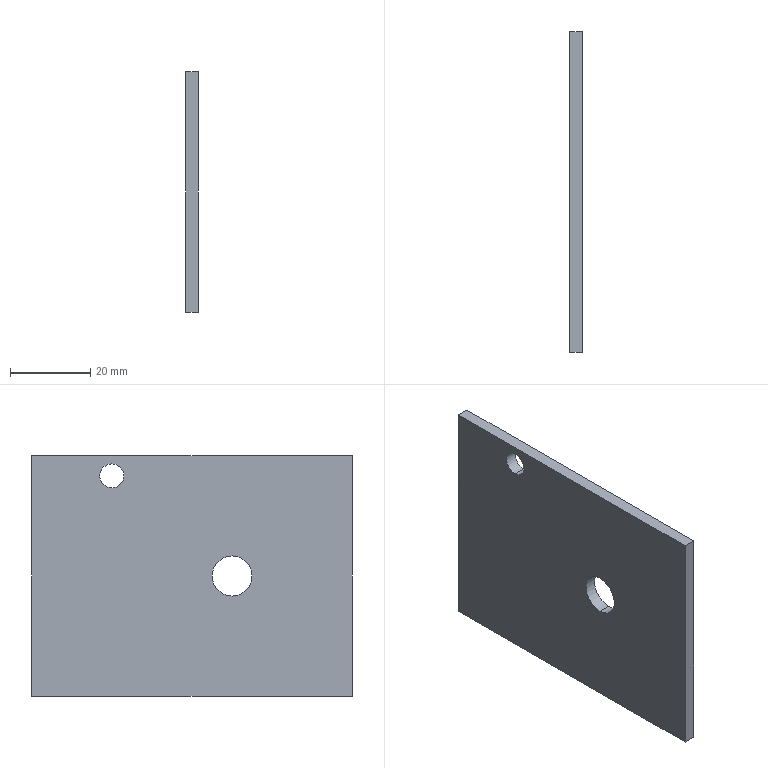Part | SolidWorks | features Extrusion 1, ICE 1 | 1 solid | 10 faces | box 3 x 80 x 60 mm | volume 14080 mm3 | plane 6 | cylinder 4 | commonest cylinder face diameters 6 x2 10 x2
STEP:
#1=CARTESIAN_POINT('',(0.,-10.,5.));
#2=VERTEX_POINT('',#1);
#3=CARTESIAN_POINT('',(0.,-10.,-5.));
#4=VERTEX_POINT('',#3);
#5=CARTESIAN_POINT('',(0.,-10.,0.));
#6=DIRECTION('',(1.,0.,0.));
#7=DIRECTION('',(0.,0.,-1.));
#8=AXIS2_PLACEMENT_3D('',#5,#6,#7);
#9=CIRCLE('',#8,5.);
#10=EDGE_CURVE('',#2,#4,#9,.T.);
#11=ORIENTED_EDGE('',*,*,#10,.F.);
#12=CARTESIAN_POINT('',(3.,-10.,5.));
#13=VERTEX_POINT('',#12);
#14=CARTESIAN_POINT('',(0.,-10.,5.));
#15=DIRECTION('',(1.,0.,0.));
#16=VECTOR('',#15,1000.);
#17=LINE('',#14,#16);
#18=EDGE_CURVE('',#2,#13,#17,.T.);
#19=ORIENTED_EDGE('',*,*,#18,.T.);
#20=CARTESIAN_POINT('',(3.,-10.,-5.));
#21=VERTEX_POINT('',#20);
#22=CARTESIAN_POINT('',(3.,-10.,0.));
#23=DIRECTION('',(1.,0.,0.));
#24=DIRECTION('',(0.,0.,-1.));
#25=AXIS2_PLACEMENT_3D('',#22,#23,#24);
#26=CIRCLE('',#25,5.);
#27=EDGE_CURVE('',#13,#21,#26,.T.);
#28=ORIENTED_EDGE('',*,*,#27,.T.);
#29=CARTESIAN_POINT('',(0.,-10.,-5.));
#30=DIRECTION('',(1.,0.,0.));
#31=VECTOR('',#30,1000.);
#32=LINE('',#29,#31);
#33=EDGE_CURVE('',#4,#21,#32,.T.);
#34=ORIENTED_EDGE('',*,*,#33,.F.);
#35=EDGE_LOOP('',(#11,#19,#28,#34));
#36=FACE_OUTER_BOUND('',#35,.T.);
#37=CARTESIAN_POINT('',(0.,-10.,0.));
#38=DIRECTION('',(1.,0.,0.));
#39=DIRECTION('',(0.,0.,-1.));
#40=AXIS2_PLACEMENT_3D('',#37,#38,#39);
#41=CYLINDRICAL_SURFACE('',#40,5.);
#42=ADVANCED_FACE('',(#36),#41,.F.);
#43=CARTESIAN_POINT('',(3.,20.,28.));
#44=VERTEX_POINT('',#43);
#45=CARTESIAN_POINT('',(3.,20.,22.));
#46=VERTEX_POINT('',#45);
#47=CARTESIAN_POINT('',(3.,20.,25.));
#48=DIRECTION('',(1.,0.,0.));
#49=DIRECTION('',(0.,0.,-1.));
#50=AXIS2_PLACEMENT_3D('',#47,#48,#49);
#51=CIRCLE('',#50,3.);
#52=EDGE_CURVE('',#44,#46,#51,.T.);
#53=ORIENTED_EDGE('',*,*,#52,.T.);
#54=CARTESIAN_POINT('',(0.,20.,22.));
#55=VERTEX_POINT('',#54);
#56=CARTESIAN_POINT('',(3.,20.,22.));
#57=DIRECTION('',(-1.,0.,0.));
#58=VECTOR('',#57,1000.);
#59=LINE('',#56,#58);
#60=EDGE_CURVE('',#46,#55,#59,.T.);
#61=ORIENTED_EDGE('',*,*,#60,.T.);
#62=CARTESIAN_POINT('',(0.,20.,28.));
#63=VERTEX_POINT('',#62);
#64=CARTESIAN_POINT('',(0.,20.,25.));
#65=DIRECTION('',(1.,0.,0.));
#66=DIRECTION('',(0.,0.,-1.));
#67=AXIS2_PLACEMENT_3D('',#64,#65,#66);
#68=CIRCLE('',#67,3.);
#69=EDGE_CURVE('',#63,#55,#68,.T.);
#70=ORIENTED_EDGE('',*,*,#69,.F.);
#71=CARTESIAN_POINT('',(3.,20.,28.));
#72=DIRECTION('',(-1.,0.,0.));
#73=VECTOR('',#72,1000.);
#74=LINE('',#71,#73);
#75=EDGE_CURVE('',#44,#63,#74,.T.);
#76=ORIENTED_EDGE('',*,*,#75,.F.);
#77=EDGE_LOOP('',(#53,#61,#70,#76));
#78=FACE_OUTER_BOUND('',#77,.T.);
#79=CARTESIAN_POINT('',(3.,20.,25.));
#80=DIRECTION('',(-1.,0.,0.));
#81=DIRECTION('',(0.,0.,1.));
#82=AXIS2_PLACEMENT_3D('',#79,#80,#81);
#83=CYLINDRICAL_SURFACE('',#82,3.);
#84=ADVANCED_FACE('',(#78),#83,.F.);
#85=CARTESIAN_POINT('',(3.,-10.,0.));
#86=DIRECTION('',(1.,0.,0.));
#87=DIRECTION('',(0.,0.,-1.));
#88=AXIS2_PLACEMENT_3D('',#85,#86,#87);
#89=CIRCLE('',#88,5.);
#90=EDGE_CURVE('',#21,#13,#89,.T.);
#91=ORIENTED_EDGE('',*,*,#90,.F.);
#92=ORIENTED_EDGE('',*,*,#27,.F.);
#93=EDGE_LOOP('',(#91,#92));
#94=FACE_BOUND('',#93,.T.);
#95=CARTESIAN_POINT('',(3.,-40.,-30.));
#96=VERTEX_POINT('',#95);
#97=CARTESIAN_POINT('',(3.,40.,-30.));
#98=VERTEX_POINT('',#97);
#99=CARTESIAN_POINT('',(3.,-40.,-30.));
#100=DIRECTION('',(0.,1.,0.));
#101=VECTOR('',#100,1000.);
#102=LINE('',#99,#101);
#103=EDGE_CURVE('',#96,#98,#102,.T.);
#104=ORIENTED_EDGE('',*,*,#103,.T.);
#105=CARTESIAN_POINT('',(3.,40.,30.));
#106=VERTEX_POINT('',#105);
#107=CARTESIAN_POINT('',(3.,40.,30.));
#108=DIRECTION('',(0.,0.,1.));
#109=VECTOR('',#108,1000.);
#110=LINE('',#107,#109);
#111=EDGE_CURVE('',#98,#106,#110,.T.);
#112=ORIENTED_EDGE('',*,*,#111,.T.);
#113=CARTESIAN_POINT('',(3.,-40.,30.));
#114=VERTEX_POINT('',#113);
#115=CARTESIAN_POINT('',(3.,-40.,30.));
#116=DIRECTION('',(0.,-1.,0.));
#117=VECTOR('',#116,1000.);
#118=LINE('',#115,#117);
#119=EDGE_CURVE('',#106,#114,#118,.T.);
#120=ORIENTED_EDGE('',*,*,#119,.T.);
#121=CARTESIAN_POINT('',(3.,-40.,30.));
#122=DIRECTION('',(0.,0.,-1.));
#123=VECTOR('',#122,1000.);
#124=LINE('',#121,#123);
#125=EDGE_CURVE('',#114,#96,#124,.T.);
#126=ORIENTED_EDGE('',*,*,#125,.T.);
#127=EDGE_LOOP('',(#104,#112,#120,#126));
#128=FACE_OUTER_BOUND('',#127,.T.);
#129=ORIENTED_EDGE('',*,*,#52,.F.);
#130=CARTESIAN_POINT('',(3.,20.,25.));
#131=DIRECTION('',(1.,0.,0.));
#132=DIRECTION('',(0.,0.,-1.));
#133=AXIS2_PLACEMENT_3D('',#130,#131,#132);
#134=CIRCLE('',#133,3.);
#135=EDGE_CURVE('',#46,#44,#134,.T.);
#136=ORIENTED_EDGE('',*,*,#135,.F.);
#137=EDGE_LOOP('',(#129,#136));
#138=FACE_BOUND('',#137,.T.);
#139=CARTESIAN_POINT('',(3.,0.,0.));
#140=DIRECTION('',(-1.,0.,0.));
#141=DIRECTION('',(0.,0.,1.));
#142=AXIS2_PLACEMENT_3D('',#139,#140,#141);
#143=PLANE('',#142);
#144=ADVANCED_FACE('',(#94,#128,#138),#143,.F.);
#145=CARTESIAN_POINT('',(0.,-10.,0.));
#146=DIRECTION('',(1.,0.,0.));
#147=DIRECTION('',(0.,0.,-1.));
#148=AXIS2_PLACEMENT_3D('',#145,#146,#147);
#149=CIRCLE('',#148,5.);
#150=EDGE_CURVE('',#4,#2,#149,.T.);
#151=ORIENTED_EDGE('',*,*,#150,.T.);
#152=ORIENTED_EDGE('',*,*,#10,.T.);
#153=EDGE_LOOP('',(#151,#152));
#154=FACE_BOUND('',#153,.T.);
#155=ORIENTED_EDGE('',*,*,#69,.T.);
#156=CARTESIAN_POINT('',(0.,20.,25.));
#157=DIRECTION('',(1.,0.,0.));
#158=DIRECTION('',(0.,0.,-1.));
#159=AXIS2_PLACEMENT_3D('',#156,#157,#158);
#160=CIRCLE('',#159,3.);
#161=EDGE_CURVE('',#55,#63,#160,.T.);
#162=ORIENTED_EDGE('',*,*,#161,.T.);
#163=EDGE_LOOP('',(#155,#162));
#164=FACE_BOUND('',#163,.T.);
#165=CARTESIAN_POINT('',(0.,-40.,-30.));
#166=VERTEX_POINT('',#165);
#167=CARTESIAN_POINT('',(0.,40.,-30.));
#168=VERTEX_POINT('',#167);
#169=CARTESIAN_POINT('',(0.,-40.,-30.));
#170=DIRECTION('',(0.,1.,0.));
#171=VECTOR('',#170,1000.);
#172=LINE('',#169,#171);
#173=EDGE_CURVE('',#166,#168,#172,.T.);
#174=ORIENTED_EDGE('',*,*,#173,.F.);
#175=CARTESIAN_POINT('',(0.,-40.,30.));
#176=VERTEX_POINT('',#175);
#177=CARTESIAN_POINT('',(0.,-40.,30.));
#178=DIRECTION('',(0.,0.,-1.));
#179=VECTOR('',#178,1000.);
#180=LINE('',#177,#179);
#181=EDGE_CURVE('',#176,#166,#180,.T.);
#182=ORIENTED_EDGE('',*,*,#181,.F.);
#183=CARTESIAN_POINT('',(0.,40.,30.));
#184=VERTEX_POINT('',#183);
#185=CARTESIAN_POINT('',(0.,-40.,30.));
#186=DIRECTION('',(0.,-1.,0.));
#187=VECTOR('',#186,1000.);
#188=LINE('',#185,#187);
#189=EDGE_CURVE('',#184,#176,#188,.T.);
#190=ORIENTED_EDGE('',*,*,#189,.F.);
#191=CARTESIAN_POINT('',(0.,40.,30.));
#192=DIRECTION('',(0.,0.,1.));
#193=VECTOR('',#192,1000.);
#194=LINE('',#191,#193);
#195=EDGE_CURVE('',#168,#184,#194,.T.);
#196=ORIENTED_EDGE('',*,*,#195,.F.);
#197=EDGE_LOOP('',(#174,#182,#190,#196));
#198=FACE_OUTER_BOUND('',#197,.T.);
#199=CARTESIAN_POINT('',(0.,0.,0.));
#200=DIRECTION('',(-1.,0.,0.));
#201=DIRECTION('',(0.,0.,1.));
#202=AXIS2_PLACEMENT_3D('',#199,#200,#201);
#203=PLANE('',#202);
#204=ADVANCED_FACE('',(#154,#164,#198),#203,.T.);
#205=ORIENTED_EDGE('',*,*,#173,.T.);
#206=CARTESIAN_POINT('',(3.,40.,-30.));
#207=DIRECTION('',(-1.,0.,0.));
#208=VECTOR('',#207,1000.);
#209=LINE('',#206,#208);
#210=EDGE_CURVE('',#98,#168,#209,.T.);
#211=ORIENTED_EDGE('',*,*,#210,.F.);
#212=ORIENTED_EDGE('',*,*,#103,.F.);
#213=CARTESIAN_POINT('',(3.,-40.,-30.));
#214=DIRECTION('',(-1.,0.,0.));
#215=VECTOR('',#214,1000.);
#216=LINE('',#213,#215);
#217=EDGE_CURVE('',#96,#166,#216,.T.);
#218=ORIENTED_EDGE('',*,*,#217,.T.);
#219=EDGE_LOOP('',(#205,#211,#212,#218));
#220=FACE_OUTER_BOUND('',#219,.T.);
#221=CARTESIAN_POINT('',(3.,-40.,-30.));
#222=DIRECTION('',(0.,0.,1.));
#223=DIRECTION('',(1.,0.,0.));
#224=AXIS2_PLACEMENT_3D('',#221,#222,#223);
#225=PLANE('',#224);
#226=ADVANCED_FACE('',(#220),#225,.F.);
#227=ORIENTED_EDGE('',*,*,#195,.T.);
#228=CARTESIAN_POINT('',(3.,40.,30.));
#229=DIRECTION('',(-1.,0.,0.));
#230=VECTOR('',#229,1000.);
#231=LINE('',#228,#230);
#232=EDGE_CURVE('',#106,#184,#231,.T.);
#233=ORIENTED_EDGE('',*,*,#232,.F.);
#234=ORIENTED_EDGE('',*,*,#111,.F.);
#235=ORIENTED_EDGE('',*,*,#210,.T.);
#236=EDGE_LOOP('',(#227,#233,#234,#235));
#237=FACE_OUTER_BOUND('',#236,.T.);
#238=CARTESIAN_POINT('',(3.,40.,30.));
#239=DIRECTION('',(0.,-1.,0.));
#240=DIRECTION('',(0.,0.,-1.));
#241=AXIS2_PLACEMENT_3D('',#238,#239,#240);
#242=PLANE('',#241);
#243=ADVANCED_FACE('',(#237),#242,.F.);
#244=ORIENTED_EDGE('',*,*,#189,.T.);
#245=CARTESIAN_POINT('',(3.,-40.,30.));
#246=DIRECTION('',(-1.,0.,0.));
#247=VECTOR('',#246,1000.);
#248=LINE('',#245,#247);
#249=EDGE_CURVE('',#114,#176,#248,.T.);
#250=ORIENTED_EDGE('',*,*,#249,.F.);
#251=ORIENTED_EDGE('',*,*,#119,.F.);
#252=ORIENTED_EDGE('',*,*,#232,.T.);
#253=EDGE_LOOP('',(#244,#250,#251,#252));
#254=FACE_OUTER_BOUND('',#253,.T.);
#255=CARTESIAN_POINT('',(3.,-40.,30.));
#256=DIRECTION('',(0.,0.,-1.));
#257=DIRECTION('',(-1.,0.,0.));
#258=AXIS2_PLACEMENT_3D('',#255,#256,#257);
#259=PLANE('',#258);
#260=ADVANCED_FACE('',(#254),#259,.F.);
#261=ORIENTED_EDGE('',*,*,#181,.T.);
#262=ORIENTED_EDGE('',*,*,#217,.F.);
#263=ORIENTED_EDGE('',*,*,#125,.F.);
#264=ORIENTED_EDGE('',*,*,#249,.T.);
#265=EDGE_LOOP('',(#261,#262,#263,#264));
#266=FACE_OUTER_BOUND('',#265,.T.);
#267=CARTESIAN_POINT('',(3.,-40.,30.));
#268=DIRECTION('',(0.,1.,0.));
#269=DIRECTION('',(0.,0.,1.));
#270=AXIS2_PLACEMENT_3D('',#267,#268,#269);
#271=PLANE('',#270);
#272=ADVANCED_FACE('',(#266),#271,.F.);
#273=ORIENTED_EDGE('',*,*,#60,.F.);
#274=ORIENTED_EDGE('',*,*,#135,.T.);
#275=ORIENTED_EDGE('',*,*,#75,.T.);
#276=ORIENTED_EDGE('',*,*,#161,.F.);
#277=EDGE_LOOP('',(#273,#274,#275,#276));
#278=FACE_OUTER_BOUND('',#277,.T.);
#279=CARTESIAN_POINT('',(3.,20.,25.));
#280=DIRECTION('',(-1.,0.,0.));
#281=DIRECTION('',(0.,0.,1.));
#282=AXIS2_PLACEMENT_3D('',#279,#280,#281);
#283=CYLINDRICAL_SURFACE('',#282,3.);
#284=ADVANCED_FACE('',(#278),#283,.F.);
#285=ORIENTED_EDGE('',*,*,#18,.F.);
#286=ORIENTED_EDGE('',*,*,#150,.F.);
#287=ORIENTED_EDGE('',*,*,#33,.T.);
#288=ORIENTED_EDGE('',*,*,#90,.T.);
#289=EDGE_LOOP('',(#285,#286,#287,#288));
#290=FACE_OUTER_BOUND('',#289,.T.);
#291=CARTESIAN_POINT('',(0.,-10.,0.));
#292=DIRECTION('',(1.,0.,0.));
#293=DIRECTION('',(0.,0.,-1.));
#294=AXIS2_PLACEMENT_3D('',#291,#292,#293);
#295=CYLINDRICAL_SURFACE('',#294,5.);
#296=ADVANCED_FACE('',(#290),#295,.F.);
#297=CLOSED_SHELL('',(#42,#84,#144,#204,#226,#243,#260,#272,#284,#296));
#298=MANIFOLD_SOLID_BREP('',#297);
#299=CARTESIAN_POINT('',(0.,0.,0.));
#300=DIRECTION('',(0.,0.,1.));
#301=DIRECTION('',(1.,0.,0.));
#302=AXIS2_PLACEMENT_3D('',#299,#300,#301);
#303=(LENGTH_UNIT()NAMED_UNIT(*)SI_UNIT(.MILLI.,.METRE.));
#304=UNCERTAINTY_MEASURE_WITH_UNIT(LENGTH_MEASURE(0.00001),#303,'','');
#305=(NAMED_UNIT(*)PLANE_ANGLE_UNIT()SI_UNIT($,.RADIAN.));
#306=(NAMED_UNIT(*)SI_UNIT($,.STERADIAN.)SOLID_ANGLE_UNIT());
#307=(GEOMETRIC_REPRESENTATION_CONTEXT(3)GLOBAL_UNCERTAINTY_ASSIGNED_CONTEXT((#304))GLOBAL_UNIT_ASSIGNED_CONTEXT((#303,#305,#306))REPRESENTATION_CONTEXT('',''));
#308=ADVANCED_BREP_SHAPE_REPRESENTATION('',(#298,#302),#307);